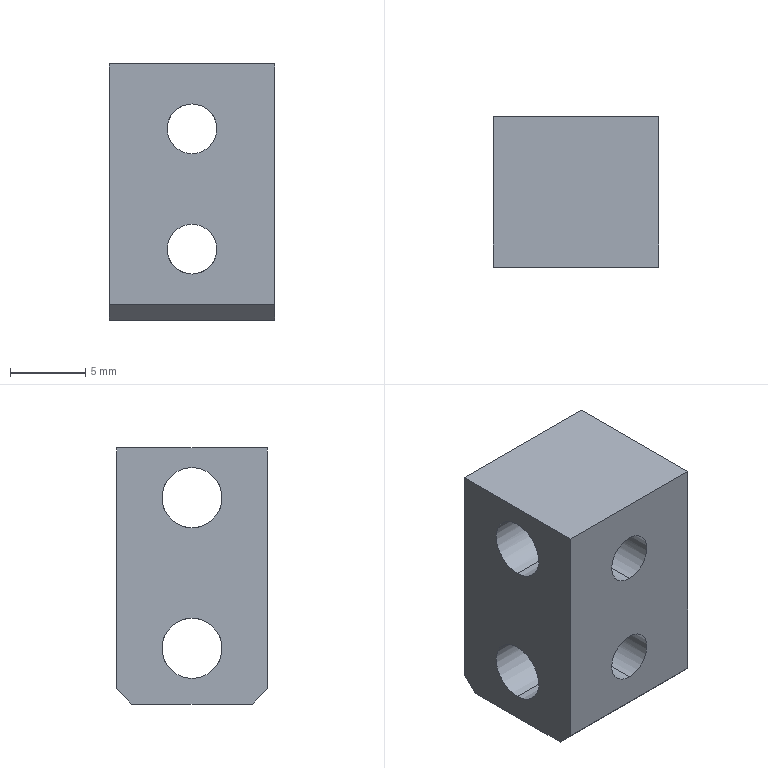Part | STEP file | 11-FG-B01611 | 1 solid | 16 faces | box 11 x 10 x 17 mm | volume 1460 mm3 | cylinder 8 | plane 8 | commonest cylinder face diameters 3.3 x4 4 x4
STEP:
#1=CARTESIAN_POINT('',(5.5,-5.,-5.45));
#2=VERTEX_POINT('',#1);
#3=CARTESIAN_POINT('',(5.5,-5.,-2.15));
#4=VERTEX_POINT('',#3);
#5=CARTESIAN_POINT('',(5.5,-5.,-3.8));
#6=DIRECTION('',(0.,1.,0.));
#7=DIRECTION('',(0.,0.,1.));
#8=AXIS2_PLACEMENT_3D('',#5,#6,#7);
#9=CIRCLE('',#8,1.65);
#10=EDGE_CURVE('',#2,#4,#9,.T.);
#11=ORIENTED_EDGE('',*,*,#10,.F.);
#12=CARTESIAN_POINT('',(5.5,-1.891,-5.45));
#13=VERTEX_POINT('',#12);
#14=CARTESIAN_POINT('',(5.5,5.,-5.45));
#15=DIRECTION('',(0.,1.,0.));
#16=VECTOR('',#15,1000.);
#17=LINE('',#14,#16);
#18=EDGE_CURVE('',#2,#13,#17,.T.);
#19=ORIENTED_EDGE('',*,*,#18,.T.);
#20=CARTESIAN_POINT('',(4.188,0.,-2.8));
#21=VERTEX_POINT('',#20);
#22=CARTESIAN_POINT('',(4.188,0.,-2.8));
#23=CARTESIAN_POINT('',(4.188,-0.1977,-2.8));
#24=CARTESIAN_POINT('',(4.163,-0.3969,-2.83));
#25=CARTESIAN_POINT('',(4.088,-0.7694,-2.944));
#26=CARTESIAN_POINT('',(4.037,-0.9458,-3.027));
#27=CARTESIAN_POINT('',(3.943,-1.267,-3.24));
#28=CARTESIAN_POINT('',(3.899,-1.413,-3.371));
#29=CARTESIAN_POINT('',(3.861,-1.602,-3.598));
#30=CARTESIAN_POINT('',(3.852,-1.66,-3.68));
#31=CARTESIAN_POINT('',(3.849,-1.763,-3.85));
#32=CARTESIAN_POINT('',(3.853,-1.807,-3.938));
#33=CARTESIAN_POINT('',(3.892,-1.922,-4.212));
#34=CARTESIAN_POINT('',(3.95,-1.968,-4.4));
#35=CARTESIAN_POINT('',(4.137,-2.007,-4.751));
#36=CARTESIAN_POINT('',(4.264,-2.001,-4.91));
#37=CARTESIAN_POINT('',(4.561,-1.97,-5.171));
#38=CARTESIAN_POINT('',(4.734,-1.944,-5.275));
#39=CARTESIAN_POINT('',(5.103,-1.905,-5.414));
#40=CARTESIAN_POINT('',(5.302,-1.891,-5.45));
#41=CARTESIAN_POINT('',(5.5,-1.891,-5.45));
#42=B_SPLINE_CURVE_WITH_KNOTS('',3,(#22,#23,#24,#25,#26,#27,#28,#29,#30,#31,#32,#33,#34,#35,#36,#37,#38,#39,#40,#41),.UNSPECIFIED.,.F.,.F.,(4,2,2,2,2,2,2,2,2,4),(0.009463,0.01005,0.01064,0.01123,0.01153,0.01182,0.01241,0.013,0.01359,0.01418),.UNSPECIFIED.);
#43=EDGE_CURVE('',#21,#13,#42,.T.);
#44=ORIENTED_EDGE('',*,*,#43,.F.);
#45=CARTESIAN_POINT('',(5.5,1.891,-5.45));
#46=VERTEX_POINT('',#45);
#47=CARTESIAN_POINT('',(5.5,1.891,-5.45));
#48=CARTESIAN_POINT('',(5.401,1.891,-5.45));
#49=CARTESIAN_POINT('',(5.3,1.895,-5.441));
#50=CARTESIAN_POINT('',(5.106,1.906,-5.405));
#51=CARTESIAN_POINT('',(5.011,1.915,-5.379));
#52=CARTESIAN_POINT('',(4.732,1.944,-5.274));
#53=CARTESIAN_POINT('',(4.562,1.97,-5.172));
#54=CARTESIAN_POINT('',(4.262,2.001,-4.909));
#55=CARTESIAN_POINT('',(4.138,2.007,-4.753));
#56=CARTESIAN_POINT('',(3.998,1.978,-4.489));
#57=CARTESIAN_POINT('',(3.96,1.962,-4.4));
#58=CARTESIAN_POINT('',(3.901,1.915,-4.217));
#59=CARTESIAN_POINT('',(3.879,1.884,-4.123));
#60=CARTESIAN_POINT('',(3.841,1.771,-3.85));
#61=CARTESIAN_POINT('',(3.848,1.666,-3.675));
#62=CARTESIAN_POINT('',(3.899,1.414,-3.372));
#63=CARTESIAN_POINT('',(3.943,1.267,-3.241));
#64=CARTESIAN_POINT('',(4.038,0.9453,-3.027));
#65=CARTESIAN_POINT('',(4.088,0.769,-2.944));
#66=CARTESIAN_POINT('',(4.163,0.398,-2.83));
#67=CARTESIAN_POINT('',(4.188,0.1981,-2.8));
#68=CARTESIAN_POINT('',(4.188,0.,-2.8));
#69=B_SPLINE_CURVE_WITH_KNOTS('',3,(#47,#48,#49,#50,#51,#52,#53,#54,#55,#56,#57,#58,#59,#60,#61,#62,#63,#64,#65,#66,#67,#68),.UNSPECIFIED.,.F.,.F.,(4,2,2,2,2,2,2,2,2,2,4),(0.004735,0.005031,0.005326,0.005917,0.006508,0.006804,0.007099,0.00769,0.008281,0.008872,0.009463),.UNSPECIFIED.);
#70=EDGE_CURVE('',#46,#21,#69,.T.);
#71=ORIENTED_EDGE('',*,*,#70,.F.);
#72=CARTESIAN_POINT('',(5.5,5.,-5.45));
#73=VERTEX_POINT('',#72);
#74=CARTESIAN_POINT('',(5.5,5.,-5.45));
#75=DIRECTION('',(0.,1.,0.));
#76=VECTOR('',#75,1000.);
#77=LINE('',#74,#76);
#78=EDGE_CURVE('',#46,#73,#77,.T.);
#79=ORIENTED_EDGE('',*,*,#78,.T.);
#80=CARTESIAN_POINT('',(5.5,5.,-2.15));
#81=VERTEX_POINT('',#80);
#82=CARTESIAN_POINT('',(5.5,5.,-3.8));
#83=DIRECTION('',(0.,1.,0.));
#84=DIRECTION('',(0.,0.,1.));
#85=AXIS2_PLACEMENT_3D('',#82,#83,#84);
#86=CIRCLE('',#85,1.65);
#87=EDGE_CURVE('',#73,#81,#86,.T.);
#88=ORIENTED_EDGE('',*,*,#87,.T.);
#89=CARTESIAN_POINT('',(5.5,5.,-2.15));
#90=DIRECTION('',(0.,1.,0.));
#91=VECTOR('',#90,1000.);
#92=LINE('',#89,#91);
#93=EDGE_CURVE('',#4,#81,#92,.T.);
#94=ORIENTED_EDGE('',*,*,#93,.F.);
#95=EDGE_LOOP('',(#11,#19,#44,#71,#79,#88,#94));
#96=FACE_OUTER_BOUND('',#95,.T.);
#97=CARTESIAN_POINT('',(5.5,5.,-3.8));
#98=DIRECTION('',(0.,1.,0.));
#99=DIRECTION('',(0.,0.,1.));
#100=AXIS2_PLACEMENT_3D('',#97,#98,#99);
#101=CYLINDRICAL_SURFACE('',#100,1.65);
#102=ADVANCED_FACE('',(#96),#101,.F.);
#103=CARTESIAN_POINT('',(5.5,-5.,2.55));
#104=VERTEX_POINT('',#103);
#105=CARTESIAN_POINT('',(5.5,-5.,5.85));
#106=VERTEX_POINT('',#105);
#107=CARTESIAN_POINT('',(5.5,-5.,4.2));
#108=DIRECTION('',(0.,1.,0.));
#109=DIRECTION('',(0.,0.,1.));
#110=AXIS2_PLACEMENT_3D('',#107,#108,#109);
#111=CIRCLE('',#110,1.65);
#112=EDGE_CURVE('',#104,#106,#111,.T.);
#113=ORIENTED_EDGE('',*,*,#112,.F.);
#114=CARTESIAN_POINT('',(5.5,5.,2.55));
#115=VERTEX_POINT('',#114);
#116=CARTESIAN_POINT('',(5.5,5.,2.55));
#117=DIRECTION('',(0.,1.,0.));
#118=VECTOR('',#117,1000.);
#119=LINE('',#116,#118);
#120=EDGE_CURVE('',#104,#115,#119,.T.);
#121=ORIENTED_EDGE('',*,*,#120,.T.);
#122=CARTESIAN_POINT('',(5.5,5.,5.85));
#123=VERTEX_POINT('',#122);
#124=CARTESIAN_POINT('',(5.5,5.,4.2));
#125=DIRECTION('',(0.,1.,0.));
#126=DIRECTION('',(0.,0.,1.));
#127=AXIS2_PLACEMENT_3D('',#124,#125,#126);
#128=CIRCLE('',#127,1.65);
#129=EDGE_CURVE('',#115,#123,#128,.T.);
#130=ORIENTED_EDGE('',*,*,#129,.T.);
#131=CARTESIAN_POINT('',(5.5,1.891,5.85));
#132=VERTEX_POINT('',#131);
#133=CARTESIAN_POINT('',(5.5,5.,5.85));
#134=DIRECTION('',(0.,1.,0.));
#135=VECTOR('',#134,1000.);
#136=LINE('',#133,#135);
#137=EDGE_CURVE('',#132,#123,#136,.T.);
#138=ORIENTED_EDGE('',*,*,#137,.F.);
#139=CARTESIAN_POINT('',(4.188,0.,3.2));
#140=VERTEX_POINT('',#139);
#141=CARTESIAN_POINT('',(4.188,0.,3.2));
#142=CARTESIAN_POINT('',(4.188,0.1976,3.2));
#143=CARTESIAN_POINT('',(4.163,0.3969,3.23));
#144=CARTESIAN_POINT('',(4.088,0.7694,3.344));
#145=CARTESIAN_POINT('',(4.037,0.9458,3.427));
#146=CARTESIAN_POINT('',(3.943,1.267,3.64));
#147=CARTESIAN_POINT('',(3.899,1.413,3.772));
#148=CARTESIAN_POINT('',(3.861,1.602,3.998));
#149=CARTESIAN_POINT('',(3.852,1.66,4.08));
#150=CARTESIAN_POINT('',(3.849,1.763,4.25));
#151=CARTESIAN_POINT('',(3.853,1.807,4.338));
#152=CARTESIAN_POINT('',(3.892,1.922,4.612));
#153=CARTESIAN_POINT('',(3.95,1.968,4.8));
#154=CARTESIAN_POINT('',(4.137,2.007,5.151));
#155=CARTESIAN_POINT('',(4.264,2.001,5.31));
#156=CARTESIAN_POINT('',(4.561,1.97,5.571));
#157=CARTESIAN_POINT('',(4.734,1.944,5.675));
#158=CARTESIAN_POINT('',(5.103,1.905,5.814));
#159=CARTESIAN_POINT('',(5.302,1.891,5.85));
#160=CARTESIAN_POINT('',(5.5,1.891,5.85));
#161=B_SPLINE_CURVE_WITH_KNOTS('',3,(#141,#142,#143,#144,#145,#146,#147,#148,#149,#150,#151,#152,#153,#154,#155,#156,#157,#158,#159,#160),.UNSPECIFIED.,.F.,.F.,(4,2,2,2,2,2,2,2,2,4),(0.004745,0.005336,0.005928,0.00652,0.006816,0.007112,0.007703,0.008295,0.008887,0.009479),.UNSPECIFIED.);
#162=EDGE_CURVE('',#140,#132,#161,.T.);
#163=ORIENTED_EDGE('',*,*,#162,.F.);
#164=CARTESIAN_POINT('',(5.5,-1.891,5.85));
#165=VERTEX_POINT('',#164);
#166=CARTESIAN_POINT('',(5.5,-1.891,5.85));
#167=CARTESIAN_POINT('',(5.299,-1.891,5.85));
#168=CARTESIAN_POINT('',(5.104,-1.905,5.814));
#169=CARTESIAN_POINT('',(4.825,-1.935,5.709));
#170=CARTESIAN_POINT('',(4.736,-1.946,5.666));
#171=CARTESIAN_POINT('',(4.567,-1.967,5.565));
#172=CARTESIAN_POINT('',(4.486,-1.978,5.505));
#173=CARTESIAN_POINT('',(4.337,-1.993,5.375));
#174=CARTESIAN_POINT('',(4.269,-1.999,5.303));
#175=CARTESIAN_POINT('',(4.146,-2.001,5.148));
#176=CARTESIAN_POINT('',(4.091,-1.997,5.064));
#177=CARTESIAN_POINT('',(3.998,-1.978,4.89));
#178=CARTESIAN_POINT('',(3.96,-1.962,4.8));
#179=CARTESIAN_POINT('',(3.9,-1.915,4.616));
#180=CARTESIAN_POINT('',(3.879,-1.884,4.522));
#181=CARTESIAN_POINT('',(3.841,-1.771,4.25));
#182=CARTESIAN_POINT('',(3.848,-1.665,4.075));
#183=CARTESIAN_POINT('',(3.899,-1.413,3.771));
#184=CARTESIAN_POINT('',(3.943,-1.267,3.64));
#185=CARTESIAN_POINT('',(4.037,-0.9458,3.427));
#186=CARTESIAN_POINT('',(4.088,-0.7691,3.344));
#187=CARTESIAN_POINT('',(4.163,-0.3981,3.23));
#188=CARTESIAN_POINT('',(4.188,-0.1981,3.2));
#189=CARTESIAN_POINT('',(4.188,0.,3.2));
#190=B_SPLINE_CURVE_WITH_KNOTS('',3,(#166,#167,#168,#169,#170,#171,#172,#173,#174,#175,#176,#177,#178,#179,#180,#181,#182,#183,#184,#185,#186,#187,#188,#189),.UNSPECIFIED.,.F.,.F.,(4,2,2,2,2,2,2,2,2,2,2,4),(0.,0.0005931,0.0008896,0.001186,0.001483,0.001779,0.002076,0.002372,0.002965,0.003559,0.004152,0.004745),.UNSPECIFIED.);
#191=EDGE_CURVE('',#165,#140,#190,.T.);
#192=ORIENTED_EDGE('',*,*,#191,.F.);
#193=CARTESIAN_POINT('',(5.5,5.,5.85));
#194=DIRECTION('',(0.,1.,0.));
#195=VECTOR('',#194,1000.);
#196=LINE('',#193,#195);
#197=EDGE_CURVE('',#106,#165,#196,.T.);
#198=ORIENTED_EDGE('',*,*,#197,.F.);
#199=EDGE_LOOP('',(#113,#121,#130,#138,#163,#192,#198));
#200=FACE_OUTER_BOUND('',#199,.T.);
#201=CARTESIAN_POINT('',(5.5,5.,4.2));
#202=DIRECTION('',(0.,1.,0.));
#203=DIRECTION('',(0.,0.,1.));
#204=AXIS2_PLACEMENT_3D('',#201,#202,#203);
#205=CYLINDRICAL_SURFACE('',#204,1.65);
#206=ADVANCED_FACE('',(#200),#205,.F.);
#207=CARTESIAN_POINT('',(11.,0.,7.2));
#208=VERTEX_POINT('',#207);
#209=CARTESIAN_POINT('',(11.,0.,3.2));
#210=VERTEX_POINT('',#209);
#211=CARTESIAN_POINT('',(11.,0.,5.2));
#212=DIRECTION('',(1.,0.,0.));
#213=DIRECTION('',(0.,0.,-1.));
#214=AXIS2_PLACEMENT_3D('',#211,#212,#213);
#215=CIRCLE('',#214,2.);
#216=EDGE_CURVE('',#208,#210,#215,.T.);
#217=ORIENTED_EDGE('',*,*,#216,.T.);
#218=CARTESIAN_POINT('',(6.812,0.,3.2));
#219=VERTEX_POINT('',#218);
#220=CARTESIAN_POINT('',(15.,0.,3.2));
#221=DIRECTION('',(-1.,0.,0.));
#222=VECTOR('',#221,1000.);
#223=LINE('',#220,#222);
#224=EDGE_CURVE('',#210,#219,#223,.T.);
#225=ORIENTED_EDGE('',*,*,#224,.T.);
#226=CARTESIAN_POINT('',(6.812,0.,3.2));
#227=CARTESIAN_POINT('',(6.812,-0.09841,3.2));
#228=CARTESIAN_POINT('',(6.818,-0.1964,3.207));
#229=CARTESIAN_POINT('',(6.839,-0.3914,3.236));
#230=CARTESIAN_POINT('',(6.855,-0.4886,3.258));
#231=CARTESIAN_POINT('',(6.912,-0.7681,3.343));
#232=CARTESIAN_POINT('',(6.962,-0.945,3.427));
#233=CARTESIAN_POINT('',(7.056,-1.265,3.639));
#234=CARTESIAN_POINT('',(7.101,-1.413,3.771));
#235=CARTESIAN_POINT('',(7.152,-1.664,4.073));
#236=CARTESIAN_POINT('',(7.159,-1.769,4.247));
#237=CARTESIAN_POINT('',(7.109,-1.92,4.608));
#238=CARTESIAN_POINT('',(7.05,-1.967,4.799));
#239=CARTESIAN_POINT('',(6.911,-1.997,5.06));
#240=CARTESIAN_POINT('',(6.856,-2.001,5.145));
#241=CARTESIAN_POINT('',(6.733,-1.999,5.301));
#242=CARTESIAN_POINT('',(6.665,-1.994,5.373));
#243=CARTESIAN_POINT('',(6.44,-1.97,5.571));
#244=CARTESIAN_POINT('',(6.268,-1.944,5.674));
#245=CARTESIAN_POINT('',(5.99,-1.915,5.779));
#246=CARTESIAN_POINT('',(5.895,-1.906,5.805));
#247=CARTESIAN_POINT('',(5.7,-1.895,5.841));
#248=CARTESIAN_POINT('',(5.6,-1.891,5.85));
#249=CARTESIAN_POINT('',(5.5,-1.891,5.85));
#250=B_SPLINE_CURVE_WITH_KNOTS('',3,(#226,#227,#228,#229,#230,#231,#232,#233,#234,#235,#236,#237,#238,#239,#240,#241,#242,#243,#244,#245,#246,#247,#248,#249),.UNSPECIFIED.,.F.,.F.,(4,2,2,2,2,2,2,2,2,2,2,4),(0.01421,0.01451,0.0148,0.01539,0.01598,0.01657,0.01716,0.01746,0.01775,0.01834,0.01864,0.01893),.UNSPECIFIED.);
#251=EDGE_CURVE('',#219,#165,#250,.T.);
#252=ORIENTED_EDGE('',*,*,#251,.T.);
#253=ORIENTED_EDGE('',*,*,#191,.T.);
#254=CARTESIAN_POINT('',(0.,0.,3.2));
#255=VERTEX_POINT('',#254);
#256=CARTESIAN_POINT('',(15.,0.,3.2));
#257=DIRECTION('',(-1.,0.,0.));
#258=VECTOR('',#257,1000.);
#259=LINE('',#256,#258);
#260=EDGE_CURVE('',#140,#255,#259,.T.);
#261=ORIENTED_EDGE('',*,*,#260,.T.);
#262=CARTESIAN_POINT('',(0.,0.,7.2));
#263=VERTEX_POINT('',#262);
#264=CARTESIAN_POINT('',(0.,0.,5.2));
#265=DIRECTION('',(-1.,0.,0.));
#266=DIRECTION('',(0.,0.,1.));
#267=AXIS2_PLACEMENT_3D('',#264,#265,#266);
#268=CIRCLE('',#267,2.);
#269=EDGE_CURVE('',#255,#263,#268,.T.);
#270=ORIENTED_EDGE('',*,*,#269,.T.);
#271=CARTESIAN_POINT('',(15.,0.,7.2));
#272=DIRECTION('',(-1.,0.,0.));
#273=VECTOR('',#272,1000.);
#274=LINE('',#271,#273);
#275=EDGE_CURVE('',#208,#263,#274,.T.);
#276=ORIENTED_EDGE('',*,*,#275,.F.);
#277=EDGE_LOOP('',(#217,#225,#252,#253,#261,#270,#276));
#278=FACE_OUTER_BOUND('',#277,.T.);
#279=CARTESIAN_POINT('',(15.,0.,5.2));
#280=DIRECTION('',(-1.,0.,0.));
#281=DIRECTION('',(0.,0.,1.));
#282=AXIS2_PLACEMENT_3D('',#279,#280,#281);
#283=CYLINDRICAL_SURFACE('',#282,2.);
#284=ADVANCED_FACE('',(#278),#283,.F.);
#285=CARTESIAN_POINT('',(11.,0.,-2.8));
#286=VERTEX_POINT('',#285);
#287=CARTESIAN_POINT('',(11.,0.,-6.8));
#288=VERTEX_POINT('',#287);
#289=CARTESIAN_POINT('',(11.,0.,-4.8));
#290=DIRECTION('',(1.,0.,0.));
#291=DIRECTION('',(0.,0.,-1.));
#292=AXIS2_PLACEMENT_3D('',#289,#290,#291);
#293=CIRCLE('',#292,2.);
#294=EDGE_CURVE('',#286,#288,#293,.T.);
#295=ORIENTED_EDGE('',*,*,#294,.T.);
#296=CARTESIAN_POINT('',(0.,0.,-6.8));
#297=VERTEX_POINT('',#296);
#298=CARTESIAN_POINT('',(15.,0.,-6.8));
#299=DIRECTION('',(-1.,0.,0.));
#300=VECTOR('',#299,1000.);
#301=LINE('',#298,#300);
#302=EDGE_CURVE('',#288,#297,#301,.T.);
#303=ORIENTED_EDGE('',*,*,#302,.T.);
#304=CARTESIAN_POINT('',(0.,0.,-2.8));
#305=VERTEX_POINT('',#304);
#306=CARTESIAN_POINT('',(0.,0.,-4.8));
#307=DIRECTION('',(-1.,0.,0.));
#308=DIRECTION('',(0.,0.,1.));
#309=AXIS2_PLACEMENT_3D('',#306,#307,#308);
#310=CIRCLE('',#309,2.);
#311=EDGE_CURVE('',#297,#305,#310,.T.);
#312=ORIENTED_EDGE('',*,*,#311,.T.);
#313=CARTESIAN_POINT('',(15.,0.,-2.8));
#314=DIRECTION('',(-1.,0.,0.));
#315=VECTOR('',#314,1000.);
#316=LINE('',#313,#315);
#317=EDGE_CURVE('',#21,#305,#316,.T.);
#318=ORIENTED_EDGE('',*,*,#317,.F.);
#319=ORIENTED_EDGE('',*,*,#43,.T.);
#320=CARTESIAN_POINT('',(6.812,0.,-2.8));
#321=VERTEX_POINT('',#320);
#322=CARTESIAN_POINT('',(5.5,-1.891,-5.45));
#323=CARTESIAN_POINT('',(5.599,-1.891,-5.45));
#324=CARTESIAN_POINT('',(5.699,-1.895,-5.441));
#325=CARTESIAN_POINT('',(5.894,-1.906,-5.405));
#326=CARTESIAN_POINT('',(5.989,-1.915,-5.379));
#327=CARTESIAN_POINT('',(6.174,-1.934,-5.309));
#328=CARTESIAN_POINT('',(6.264,-1.946,-5.266));
#329=CARTESIAN_POINT('',(6.433,-1.967,-5.164));
#330=CARTESIAN_POINT('',(6.513,-1.977,-5.107));
#331=CARTESIAN_POINT('',(6.737,-2.001,-4.91));
#332=CARTESIAN_POINT('',(6.861,-2.007,-4.754));
#333=CARTESIAN_POINT('',(7.049,-1.968,-4.403));
#334=CARTESIAN_POINT('',(7.108,-1.923,-4.215));
#335=CARTESIAN_POINT('',(7.16,-1.771,-3.85));
#336=CARTESIAN_POINT('',(7.153,-1.666,-3.676));
#337=CARTESIAN_POINT('',(7.101,-1.415,-3.373));
#338=CARTESIAN_POINT('',(7.057,-1.268,-3.241));
#339=CARTESIAN_POINT('',(6.963,-0.9467,-3.028));
#340=CARTESIAN_POINT('',(6.912,-0.7697,-2.944));
#341=CARTESIAN_POINT('',(6.856,-0.4921,-2.859));
#342=CARTESIAN_POINT('',(6.84,-0.397,-2.837));
#343=CARTESIAN_POINT('',(6.818,-0.2008,-2.808));
#344=CARTESIAN_POINT('',(6.812,-0.09986,-2.8));
#345=CARTESIAN_POINT('',(6.812,0.,-2.8));
#346=B_SPLINE_CURVE_WITH_KNOTS('',3,(#322,#323,#324,#325,#326,#327,#328,#329,#330,#331,#332,#333,#334,#335,#336,#337,#338,#339,#340,#341,#342,#343,#344,#345),.UNSPECIFIED.,.F.,.F.,(4,2,2,2,2,2,2,2,2,2,2,4),(0.01418,0.01448,0.01477,0.01506,0.01536,0.01595,0.01654,0.01713,0.01772,0.01831,0.0186,0.01889),.UNSPECIFIED.);
#347=EDGE_CURVE('',#13,#321,#346,.T.);
#348=ORIENTED_EDGE('',*,*,#347,.T.);
#349=CARTESIAN_POINT('',(15.,0.,-2.8));
#350=DIRECTION('',(-1.,0.,0.));
#351=VECTOR('',#350,1000.);
#352=LINE('',#349,#351);
#353=EDGE_CURVE('',#286,#321,#352,.T.);
#354=ORIENTED_EDGE('',*,*,#353,.F.);
#355=EDGE_LOOP('',(#295,#303,#312,#318,#319,#348,#354));
#356=FACE_OUTER_BOUND('',#355,.T.);
#357=CARTESIAN_POINT('',(15.,0.,-4.8));
#358=DIRECTION('',(-1.,0.,0.));
#359=DIRECTION('',(0.,0.,1.));
#360=AXIS2_PLACEMENT_3D('',#357,#358,#359);
#361=CYLINDRICAL_SURFACE('',#360,2.);
#362=ADVANCED_FACE('',(#356),#361,.F.);
#363=CARTESIAN_POINT('',(0.,5.,8.5));
#364=VERTEX_POINT('',#363);
#365=CARTESIAN_POINT('',(0.,-5.,8.5));
#366=VERTEX_POINT('',#365);
#367=CARTESIAN_POINT('',(0.,-5.,8.5));
#368=DIRECTION('',(0.,-1.,0.));
#369=VECTOR('',#368,1000.);
#370=LINE('',#367,#369);
#371=EDGE_CURVE('',#364,#366,#370,.T.);
#372=ORIENTED_EDGE('',*,*,#371,.T.);
#373=CARTESIAN_POINT('',(11.,-5.,8.5));
#374=VERTEX_POINT('',#373);
#375=CARTESIAN_POINT('',(11.,-5.,8.5));
#376=DIRECTION('',(-1.,0.,0.));
#377=VECTOR('',#376,1000.);
#378=LINE('',#375,#377);
#379=EDGE_CURVE('',#374,#366,#378,.T.);
#380=ORIENTED_EDGE('',*,*,#379,.F.);
#381=CARTESIAN_POINT('',(11.,5.,8.5));
#382=VERTEX_POINT('',#381);
#383=CARTESIAN_POINT('',(11.,-5.,8.5));
#384=DIRECTION('',(0.,-1.,0.));
#385=VECTOR('',#384,1000.);
#386=LINE('',#383,#385);
#387=EDGE_CURVE('',#382,#374,#386,.T.);
#388=ORIENTED_EDGE('',*,*,#387,.F.);
#389=CARTESIAN_POINT('',(11.,5.,8.5));
#390=DIRECTION('',(-1.,0.,0.));
#391=VECTOR('',#390,1000.);
#392=LINE('',#389,#391);
#393=EDGE_CURVE('',#382,#364,#392,.T.);
#394=ORIENTED_EDGE('',*,*,#393,.T.);
#395=EDGE_LOOP('',(#372,#380,#388,#394));
#396=FACE_OUTER_BOUND('',#395,.T.);
#397=CARTESIAN_POINT('',(11.,-5.,8.5));
#398=DIRECTION('',(0.,0.,-1.));
#399=DIRECTION('',(-1.,0.,0.));
#400=AXIS2_PLACEMENT_3D('',#397,#398,#399);
#401=PLANE('',#400);
#402=ADVANCED_FACE('',(#396),#401,.F.);
#403=CARTESIAN_POINT('',(5.5,-5.,-3.8));
#404=DIRECTION('',(0.,1.,0.));
#405=DIRECTION('',(0.,0.,1.));
#406=AXIS2_PLACEMENT_3D('',#403,#404,#405);
#407=CIRCLE('',#406,1.65);
#408=EDGE_CURVE('',#4,#2,#407,.T.);
#409=ORIENTED_EDGE('',*,*,#408,.T.);
#410=ORIENTED_EDGE('',*,*,#10,.T.);
#411=EDGE_LOOP('',(#409,#410));
#412=FACE_BOUND('',#411,.T.);
#413=CARTESIAN_POINT('',(5.5,-5.,4.2));
#414=DIRECTION('',(0.,1.,0.));
#415=DIRECTION('',(0.,0.,1.));
#416=AXIS2_PLACEMENT_3D('',#413,#414,#415);
#417=CIRCLE('',#416,1.65);
#418=EDGE_CURVE('',#106,#104,#417,.T.);
#419=ORIENTED_EDGE('',*,*,#418,.T.);
#420=ORIENTED_EDGE('',*,*,#112,.T.);
#421=EDGE_LOOP('',(#419,#420));
#422=FACE_BOUND('',#421,.T.);
#423=CARTESIAN_POINT('',(0.,-5.,-7.5));
#424=VERTEX_POINT('',#423);
#425=CARTESIAN_POINT('',(0.,-5.,-8.5));
#426=DIRECTION('',(0.,0.,-1.));
#427=VECTOR('',#426,1000.);
#428=LINE('',#425,#427);
#429=EDGE_CURVE('',#366,#424,#428,.T.);
#430=ORIENTED_EDGE('',*,*,#429,.T.);
#431=CARTESIAN_POINT('',(11.,-5.,-7.5));
#432=VERTEX_POINT('',#431);
#433=CARTESIAN_POINT('',(11.,-5.,-7.5));
#434=DIRECTION('',(1.,0.,0.));
#435=VECTOR('',#434,1000.);
#436=LINE('',#433,#435);
#437=EDGE_CURVE('',#424,#432,#436,.T.);
#438=ORIENTED_EDGE('',*,*,#437,.T.);
#439=CARTESIAN_POINT('',(11.,-5.,-8.5));
#440=DIRECTION('',(0.,0.,-1.));
#441=VECTOR('',#440,1000.);
#442=LINE('',#439,#441);
#443=EDGE_CURVE('',#374,#432,#442,.T.);
#444=ORIENTED_EDGE('',*,*,#443,.F.);
#445=ORIENTED_EDGE('',*,*,#379,.T.);
#446=EDGE_LOOP('',(#430,#438,#444,#445));
#447=FACE_OUTER_BOUND('',#446,.T.);
#448=CARTESIAN_POINT('',(11.,-5.,-8.5));
#449=DIRECTION('',(0.,1.,0.));
#450=DIRECTION('',(0.,0.,1.));
#451=AXIS2_PLACEMENT_3D('',#448,#449,#450);
#452=PLANE('',#451);
#453=ADVANCED_FACE('',(#412,#422,#447),#452,.F.);
#454=CARTESIAN_POINT('',(0.,-4.,-8.5));
#455=VERTEX_POINT('',#454);
#456=CARTESIAN_POINT('',(0.,4.,-8.5));
#457=VERTEX_POINT('',#456);
#458=CARTESIAN_POINT('',(0.,-5.,-8.5));
#459=DIRECTION('',(0.,1.,0.));
#460=VECTOR('',#459,1000.);
#461=LINE('',#458,#460);
#462=EDGE_CURVE('',#455,#457,#461,.T.);
#463=ORIENTED_EDGE('',*,*,#462,.T.);
#464=CARTESIAN_POINT('',(11.,4.,-8.5));
#465=VERTEX_POINT('',#464);
#466=CARTESIAN_POINT('',(11.,4.,-8.5));
#467=DIRECTION('',(1.,0.,0.));
#468=VECTOR('',#467,1000.);
#469=LINE('',#466,#468);
#470=EDGE_CURVE('',#457,#465,#469,.T.);
#471=ORIENTED_EDGE('',*,*,#470,.T.);
#472=CARTESIAN_POINT('',(11.,-4.,-8.5));
#473=VERTEX_POINT('',#472);
#474=CARTESIAN_POINT('',(11.,-5.,-8.5));
#475=DIRECTION('',(0.,1.,0.));
#476=VECTOR('',#475,1000.);
#477=LINE('',#474,#476);
#478=EDGE_CURVE('',#473,#465,#477,.T.);
#479=ORIENTED_EDGE('',*,*,#478,.F.);
#480=CARTESIAN_POINT('',(11.,-4.,-8.5));
#481=DIRECTION('',(-1.,0.,0.));
#482=VECTOR('',#481,1000.);
#483=LINE('',#480,#482);
#484=EDGE_CURVE('',#473,#455,#483,.T.);
#485=ORIENTED_EDGE('',*,*,#484,.T.);
#486=EDGE_LOOP('',(#463,#471,#479,#485));
#487=FACE_OUTER_BOUND('',#486,.T.);
#488=CARTESIAN_POINT('',(11.,-5.,-8.5));
#489=DIRECTION('',(0.,0.,1.));
#490=DIRECTION('',(1.,0.,0.));
#491=AXIS2_PLACEMENT_3D('',#488,#489,#490);
#492=PLANE('',#491);
#493=ADVANCED_FACE('',(#487),#492,.F.);
#494=CARTESIAN_POINT('',(5.5,5.,-3.8));
#495=DIRECTION('',(0.,1.,0.));
#496=DIRECTION('',(0.,0.,1.));
#497=AXIS2_PLACEMENT_3D('',#494,#495,#496);
#498=CIRCLE('',#497,1.65);
#499=EDGE_CURVE('',#81,#73,#498,.T.);
#500=ORIENTED_EDGE('',*,*,#499,.F.);
#501=ORIENTED_EDGE('',*,*,#87,.F.);
#502=EDGE_LOOP('',(#500,#501));
#503=FACE_BOUND('',#502,.T.);
#504=CARTESIAN_POINT('',(5.5,5.,4.2));
#505=DIRECTION('',(0.,1.,0.));
#506=DIRECTION('',(0.,0.,1.));
#507=AXIS2_PLACEMENT_3D('',#504,#505,#506);
#508=CIRCLE('',#507,1.65);
#509=EDGE_CURVE('',#123,#115,#508,.T.);
#510=ORIENTED_EDGE('',*,*,#509,.F.);
#511=ORIENTED_EDGE('',*,*,#129,.F.);
#512=EDGE_LOOP('',(#510,#511));
#513=FACE_BOUND('',#512,.T.);
#514=CARTESIAN_POINT('',(11.,5.,-7.5));
#515=VERTEX_POINT('',#514);
#516=CARTESIAN_POINT('',(11.,5.,-8.5));
#517=DIRECTION('',(0.,0.,1.));
#518=VECTOR('',#517,1000.);
#519=LINE('',#516,#518);
#520=EDGE_CURVE('',#515,#382,#519,.T.);
#521=ORIENTED_EDGE('',*,*,#520,.F.);
#522=CARTESIAN_POINT('',(0.,5.,-7.5));
#523=VERTEX_POINT('',#522);
#524=CARTESIAN_POINT('',(11.,5.,-7.5));
#525=DIRECTION('',(-1.,0.,0.));
#526=VECTOR('',#525,1000.);
#527=LINE('',#524,#526);
#528=EDGE_CURVE('',#515,#523,#527,.T.);
#529=ORIENTED_EDGE('',*,*,#528,.T.);
#530=CARTESIAN_POINT('',(0.,5.,-8.5));
#531=DIRECTION('',(0.,0.,1.));
#532=VECTOR('',#531,1000.);
#533=LINE('',#530,#532);
#534=EDGE_CURVE('',#523,#364,#533,.T.);
#535=ORIENTED_EDGE('',*,*,#534,.T.);
#536=ORIENTED_EDGE('',*,*,#393,.F.);
#537=EDGE_LOOP('',(#521,#529,#535,#536));
#538=FACE_OUTER_BOUND('',#537,.T.);
#539=CARTESIAN_POINT('',(11.,5.,-8.5));
#540=DIRECTION('',(0.,-1.,0.));
#541=DIRECTION('',(0.,0.,-1.));
#542=AXIS2_PLACEMENT_3D('',#539,#540,#541);
#543=PLANE('',#542);
#544=ADVANCED_FACE('',(#503,#513,#538),#543,.F.);
#545=ORIENTED_EDGE('',*,*,#216,.F.);
#546=CARTESIAN_POINT('',(11.,0.,5.2));
#547=DIRECTION('',(1.,0.,0.));
#548=DIRECTION('',(0.,0.,-1.));
#549=AXIS2_PLACEMENT_3D('',#546,#547,#548);
#550=CIRCLE('',#549,2.);
#551=EDGE_CURVE('',#210,#208,#550,.T.);
#552=ORIENTED_EDGE('',*,*,#551,.F.);
#553=EDGE_LOOP('',(#545,#552));
#554=FACE_BOUND('',#553,.T.);
#555=ORIENTED_EDGE('',*,*,#294,.F.);
#556=CARTESIAN_POINT('',(11.,0.,-4.8));
#557=DIRECTION('',(1.,0.,0.));
#558=DIRECTION('',(0.,0.,-1.));
#559=AXIS2_PLACEMENT_3D('',#556,#557,#558);
#560=CIRCLE('',#559,2.);
#561=EDGE_CURVE('',#288,#286,#560,.T.);
#562=ORIENTED_EDGE('',*,*,#561,.F.);
#563=EDGE_LOOP('',(#555,#562));
#564=FACE_BOUND('',#563,.T.);
#565=ORIENTED_EDGE('',*,*,#478,.T.);
#566=CARTESIAN_POINT('',(11.,6.25,-6.25));
#567=DIRECTION('',(0.,0.7071,0.7071));
#568=VECTOR('',#567,1000.);
#569=LINE('',#566,#568);
#570=EDGE_CURVE('',#465,#515,#569,.T.);
#571=ORIENTED_EDGE('',*,*,#570,.T.);
#572=ORIENTED_EDGE('',*,*,#520,.T.);
#573=ORIENTED_EDGE('',*,*,#387,.T.);
#574=ORIENTED_EDGE('',*,*,#443,.T.);
#575=CARTESIAN_POINT('',(11.,-6.25,-6.25));
#576=DIRECTION('',(0.,0.7071,-0.7071));
#577=VECTOR('',#576,1000.);
#578=LINE('',#575,#577);
#579=EDGE_CURVE('',#432,#473,#578,.T.);
#580=ORIENTED_EDGE('',*,*,#579,.T.);
#581=EDGE_LOOP('',(#565,#571,#572,#573,#574,#580));
#582=FACE_OUTER_BOUND('',#581,.T.);
#583=CARTESIAN_POINT('',(11.,0.,0.));
#584=DIRECTION('',(1.,0.,0.));
#585=DIRECTION('',(0.,0.,-1.));
#586=AXIS2_PLACEMENT_3D('',#583,#584,#585);
#587=PLANE('',#586);
#588=ADVANCED_FACE('',(#554,#564,#582),#587,.T.);
#589=CARTESIAN_POINT('',(0.,0.,5.2));
#590=DIRECTION('',(-1.,0.,0.));
#591=DIRECTION('',(0.,0.,1.));
#592=AXIS2_PLACEMENT_3D('',#589,#590,#591);
#593=CIRCLE('',#592,2.);
#594=EDGE_CURVE('',#263,#255,#593,.T.);
#595=ORIENTED_EDGE('',*,*,#594,.F.);
#596=ORIENTED_EDGE('',*,*,#269,.F.);
#597=EDGE_LOOP('',(#595,#596));
#598=FACE_BOUND('',#597,.T.);
#599=CARTESIAN_POINT('',(0.,0.,-4.8));
#600=DIRECTION('',(-1.,0.,0.));
#601=DIRECTION('',(0.,0.,1.));
#602=AXIS2_PLACEMENT_3D('',#599,#600,#601);
#603=CIRCLE('',#602,2.);
#604=EDGE_CURVE('',#305,#297,#603,.T.);
#605=ORIENTED_EDGE('',*,*,#604,.F.);
#606=ORIENTED_EDGE('',*,*,#311,.F.);
#607=EDGE_LOOP('',(#605,#606));
#608=FACE_BOUND('',#607,.T.);
#609=ORIENTED_EDGE('',*,*,#534,.F.);
#610=CARTESIAN_POINT('',(0.,5.,-7.5));
#611=DIRECTION('',(0.,-0.7071,-0.7071));
#612=VECTOR('',#611,1000.);
#613=LINE('',#610,#612);
#614=EDGE_CURVE('',#523,#457,#613,.T.);
#615=ORIENTED_EDGE('',*,*,#614,.T.);
#616=ORIENTED_EDGE('',*,*,#462,.F.);
#617=CARTESIAN_POINT('',(0.,-4.,-8.5));
#618=DIRECTION('',(0.,-0.7071,0.7071));
#619=VECTOR('',#618,1000.);
#620=LINE('',#617,#619);
#621=EDGE_CURVE('',#455,#424,#620,.T.);
#622=ORIENTED_EDGE('',*,*,#621,.T.);
#623=ORIENTED_EDGE('',*,*,#429,.F.);
#624=ORIENTED_EDGE('',*,*,#371,.F.);
#625=EDGE_LOOP('',(#609,#615,#616,#622,#623,#624));
#626=FACE_OUTER_BOUND('',#625,.T.);
#627=CARTESIAN_POINT('',(0.,0.,0.));
#628=DIRECTION('',(1.,0.,0.));
#629=DIRECTION('',(0.,0.,-1.));
#630=AXIS2_PLACEMENT_3D('',#627,#628,#629);
#631=PLANE('',#630);
#632=ADVANCED_FACE('',(#598,#608,#626),#631,.F.);
#633=ORIENTED_EDGE('',*,*,#302,.F.);
#634=ORIENTED_EDGE('',*,*,#561,.T.);
#635=ORIENTED_EDGE('',*,*,#353,.T.);
#636=CARTESIAN_POINT('',(6.812,0.,-2.8));
#637=CARTESIAN_POINT('',(6.812,0.2006,-2.8));
#638=CARTESIAN_POINT('',(6.836,0.3943,-2.829));
#639=CARTESIAN_POINT('',(6.912,0.7702,-2.944));
#640=CARTESIAN_POINT('',(6.962,0.9438,-3.026));
#641=CARTESIAN_POINT('',(7.057,1.268,-3.241));
#642=CARTESIAN_POINT('',(7.1,1.411,-3.369));
#643=CARTESIAN_POINT('',(7.139,1.6,-3.596));
#644=CARTESIAN_POINT('',(7.148,1.659,-3.678));
#645=CARTESIAN_POINT('',(7.151,1.761,-3.848));
#646=CARTESIAN_POINT('',(7.147,1.806,-3.936));
#647=CARTESIAN_POINT('',(7.121,1.883,-4.12));
#648=CARTESIAN_POINT('',(7.101,1.914,-4.212));
#649=CARTESIAN_POINT('',(7.042,1.961,-4.395));
#650=CARTESIAN_POINT('',(7.003,1.977,-4.487));
#651=CARTESIAN_POINT('',(6.864,2.007,-4.75));
#652=CARTESIAN_POINT('',(6.737,2.001,-4.909));
#653=CARTESIAN_POINT('',(6.44,1.97,-5.171));
#654=CARTESIAN_POINT('',(6.267,1.944,-5.274));
#655=CARTESIAN_POINT('',(5.99,1.915,-5.379));
#656=CARTESIAN_POINT('',(5.893,1.906,-5.406));
#657=CARTESIAN_POINT('',(5.698,1.895,-5.441));
#658=CARTESIAN_POINT('',(5.599,1.891,-5.45));
#659=CARTESIAN_POINT('',(5.5,1.891,-5.45));
#660=B_SPLINE_CURVE_WITH_KNOTS('',3,(#636,#637,#638,#639,#640,#641,#642,#643,#644,#645,#646,#647,#648,#649,#650,#651,#652,#653,#654,#655,#656,#657,#658,#659),.UNSPECIFIED.,.F.,.F.,(4,2,2,2,2,2,2,2,2,2,2,4),(0.,0.0005919,0.001184,0.001776,0.002072,0.002368,0.002664,0.00296,0.003551,0.004143,0.004439,0.004735),.UNSPECIFIED.);
#661=EDGE_CURVE('',#321,#46,#660,.T.);
#662=ORIENTED_EDGE('',*,*,#661,.T.);
#663=ORIENTED_EDGE('',*,*,#70,.T.);
#664=ORIENTED_EDGE('',*,*,#317,.T.);
#665=ORIENTED_EDGE('',*,*,#604,.T.);
#666=EDGE_LOOP('',(#633,#634,#635,#662,#663,#664,#665));
#667=FACE_OUTER_BOUND('',#666,.T.);
#668=CARTESIAN_POINT('',(15.,0.,-4.8));
#669=DIRECTION('',(-1.,0.,0.));
#670=DIRECTION('',(0.,0.,1.));
#671=AXIS2_PLACEMENT_3D('',#668,#669,#670);
#672=CYLINDRICAL_SURFACE('',#671,2.);
#673=ADVANCED_FACE('',(#667),#672,.F.);
#674=ORIENTED_EDGE('',*,*,#224,.F.);
#675=ORIENTED_EDGE('',*,*,#551,.T.);
#676=ORIENTED_EDGE('',*,*,#275,.T.);
#677=ORIENTED_EDGE('',*,*,#594,.T.);
#678=ORIENTED_EDGE('',*,*,#260,.F.);
#679=ORIENTED_EDGE('',*,*,#162,.T.);
#680=CARTESIAN_POINT('',(5.5,1.891,5.85));
#681=CARTESIAN_POINT('',(5.599,1.891,5.85));
#682=CARTESIAN_POINT('',(5.699,1.895,5.841));
#683=CARTESIAN_POINT('',(5.894,1.906,5.805));
#684=CARTESIAN_POINT('',(5.989,1.915,5.779));
#685=CARTESIAN_POINT('',(6.174,1.934,5.709));
#686=CARTESIAN_POINT('',(6.265,1.946,5.665));
#687=CARTESIAN_POINT('',(6.433,1.967,5.564));
#688=CARTESIAN_POINT('',(6.513,1.978,5.506));
#689=CARTESIAN_POINT('',(6.737,2.001,5.31));
#690=CARTESIAN_POINT('',(6.861,2.007,5.153));
#691=CARTESIAN_POINT('',(7.049,1.968,4.802));
#692=CARTESIAN_POINT('',(7.108,1.923,4.614));
#693=CARTESIAN_POINT('',(7.16,1.77,4.249));
#694=CARTESIAN_POINT('',(7.152,1.665,4.075));
#695=CARTESIAN_POINT('',(7.101,1.414,3.772));
#696=CARTESIAN_POINT('',(7.056,1.266,3.64));
#697=CARTESIAN_POINT('',(6.962,0.9451,3.427));
#698=CARTESIAN_POINT('',(6.912,0.7679,3.343));
#699=CARTESIAN_POINT('',(6.837,0.3976,3.23));
#700=CARTESIAN_POINT('',(6.812,0.1972,3.2));
#701=CARTESIAN_POINT('',(6.812,0.,3.2));
#702=B_SPLINE_CURVE_WITH_KNOTS('',3,(#680,#681,#682,#683,#684,#685,#686,#687,#688,#689,#690,#691,#692,#693,#694,#695,#696,#697,#698,#699,#700,#701),.UNSPECIFIED.,.F.,.F.,(4,2,2,2,2,2,2,2,2,2,4),(0.009479,0.009774,0.01007,0.01037,0.01066,0.01125,0.01184,0.01244,0.01303,0.01362,0.01421),.UNSPECIFIED.);
#703=EDGE_CURVE('',#132,#219,#702,.T.);
#704=ORIENTED_EDGE('',*,*,#703,.T.);
#705=EDGE_LOOP('',(#674,#675,#676,#677,#678,#679,#704));
#706=FACE_OUTER_BOUND('',#705,.T.);
#707=CARTESIAN_POINT('',(15.,0.,5.2));
#708=DIRECTION('',(-1.,0.,0.));
#709=DIRECTION('',(0.,0.,1.));
#710=AXIS2_PLACEMENT_3D('',#707,#708,#709);
#711=CYLINDRICAL_SURFACE('',#710,2.);
#712=ADVANCED_FACE('',(#706),#711,.F.);
#713=ORIENTED_EDGE('',*,*,#570,.F.);
#714=ORIENTED_EDGE('',*,*,#470,.F.);
#715=ORIENTED_EDGE('',*,*,#614,.F.);
#716=ORIENTED_EDGE('',*,*,#528,.F.);
#717=EDGE_LOOP('',(#713,#714,#715,#716));
#718=FACE_OUTER_BOUND('',#717,.T.);
#719=CARTESIAN_POINT('',(11.,5.,-7.5));
#720=DIRECTION('',(0.,-0.7071,0.7071));
#721=DIRECTION('',(-1.,0.,0.));
#722=AXIS2_PLACEMENT_3D('',#719,#720,#721);
#723=PLANE('',#722);
#724=ADVANCED_FACE('',(#718),#723,.F.);
#725=ORIENTED_EDGE('',*,*,#579,.F.);
#726=ORIENTED_EDGE('',*,*,#437,.F.);
#727=ORIENTED_EDGE('',*,*,#621,.F.);
#728=ORIENTED_EDGE('',*,*,#484,.F.);
#729=EDGE_LOOP('',(#725,#726,#727,#728));
#730=FACE_OUTER_BOUND('',#729,.T.);
#731=CARTESIAN_POINT('',(11.,-4.,-8.5));
#732=DIRECTION('',(0.,0.7071,0.7071));
#733=DIRECTION('',(-1.,0.,0.));
#734=AXIS2_PLACEMENT_3D('',#731,#732,#733);
#735=PLANE('',#734);
#736=ADVANCED_FACE('',(#730),#735,.F.);
#737=ORIENTED_EDGE('',*,*,#120,.F.);
#738=ORIENTED_EDGE('',*,*,#418,.F.);
#739=ORIENTED_EDGE('',*,*,#197,.T.);
#740=ORIENTED_EDGE('',*,*,#251,.F.);
#741=ORIENTED_EDGE('',*,*,#703,.F.);
#742=ORIENTED_EDGE('',*,*,#137,.T.);
#743=ORIENTED_EDGE('',*,*,#509,.T.);
#744=EDGE_LOOP('',(#737,#738,#739,#740,#741,#742,#743));
#745=FACE_OUTER_BOUND('',#744,.T.);
#746=CARTESIAN_POINT('',(5.5,5.,4.2));
#747=DIRECTION('',(0.,1.,0.));
#748=DIRECTION('',(0.,0.,1.));
#749=AXIS2_PLACEMENT_3D('',#746,#747,#748);
#750=CYLINDRICAL_SURFACE('',#749,1.65);
#751=ADVANCED_FACE('',(#745),#750,.F.);
#752=ORIENTED_EDGE('',*,*,#18,.F.);
#753=ORIENTED_EDGE('',*,*,#408,.F.);
#754=ORIENTED_EDGE('',*,*,#93,.T.);
#755=ORIENTED_EDGE('',*,*,#499,.T.);
#756=ORIENTED_EDGE('',*,*,#78,.F.);
#757=ORIENTED_EDGE('',*,*,#661,.F.);
#758=ORIENTED_EDGE('',*,*,#347,.F.);
#759=EDGE_LOOP('',(#752,#753,#754,#755,#756,#757,#758));
#760=FACE_OUTER_BOUND('',#759,.T.);
#761=CARTESIAN_POINT('',(5.5,5.,-3.8));
#762=DIRECTION('',(0.,1.,0.));
#763=DIRECTION('',(0.,0.,1.));
#764=AXIS2_PLACEMENT_3D('',#761,#762,#763);
#765=CYLINDRICAL_SURFACE('',#764,1.65);
#766=ADVANCED_FACE('',(#760),#765,.F.);
#767=CLOSED_SHELL('',(#102,#206,#284,#362,#402,#453,#493,#544,#588,#632,#673,#712,#724,#736,#751,#766));
#768=MANIFOLD_SOLID_BREP('',#767);
#769=CARTESIAN_POINT('',(0.,0.,0.));
#770=DIRECTION('',(0.,0.,1.));
#771=DIRECTION('',(1.,0.,0.));
#772=AXIS2_PLACEMENT_3D('',#769,#770,#771);
#773=(LENGTH_UNIT()NAMED_UNIT(*)SI_UNIT(.MILLI.,.METRE.));
#774=UNCERTAINTY_MEASURE_WITH_UNIT(LENGTH_MEASURE(0.00001),#773,'','');
#775=(NAMED_UNIT(*)PLANE_ANGLE_UNIT()SI_UNIT($,.RADIAN.));
#776=(NAMED_UNIT(*)SI_UNIT($,.STERADIAN.)SOLID_ANGLE_UNIT());
#777=(GEOMETRIC_REPRESENTATION_CONTEXT(3)GLOBAL_UNCERTAINTY_ASSIGNED_CONTEXT((#774))GLOBAL_UNIT_ASSIGNED_CONTEXT((#773,#775,#776))REPRESENTATION_CONTEXT('',''));
#778=ADVANCED_BREP_SHAPE_REPRESENTATION('',(#768,#772),#777);